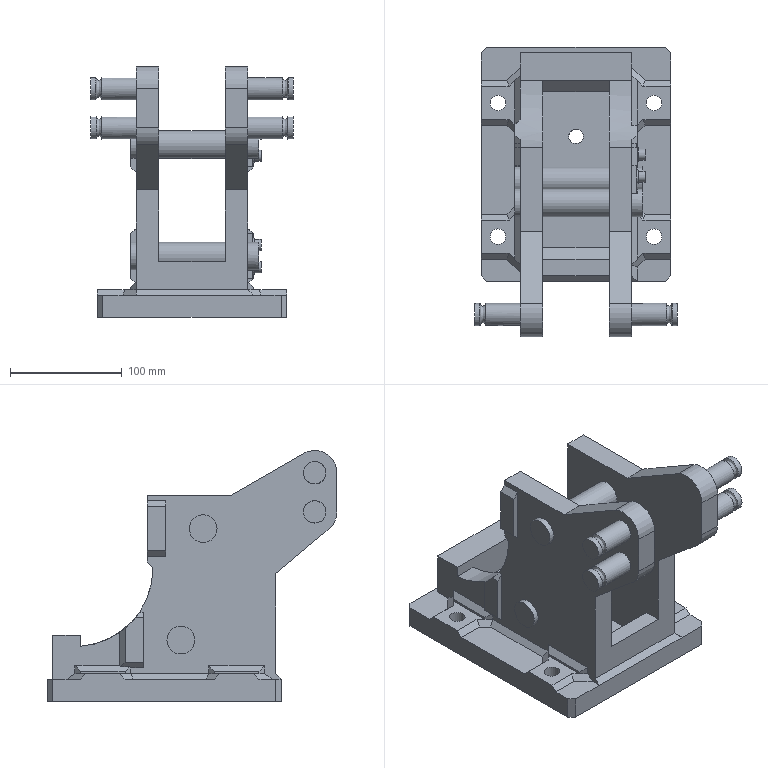Part | NX | features solid 2 | 1 solid | 167 faces | box 182 x 260 x 225 mm | volume 2059506 mm3 | plane 129 | cylinder 34 | spline 4 | commonest cylinder face diameters 20 x8 25 x6 10 x4 12.2 x4 14 x4 40 x4